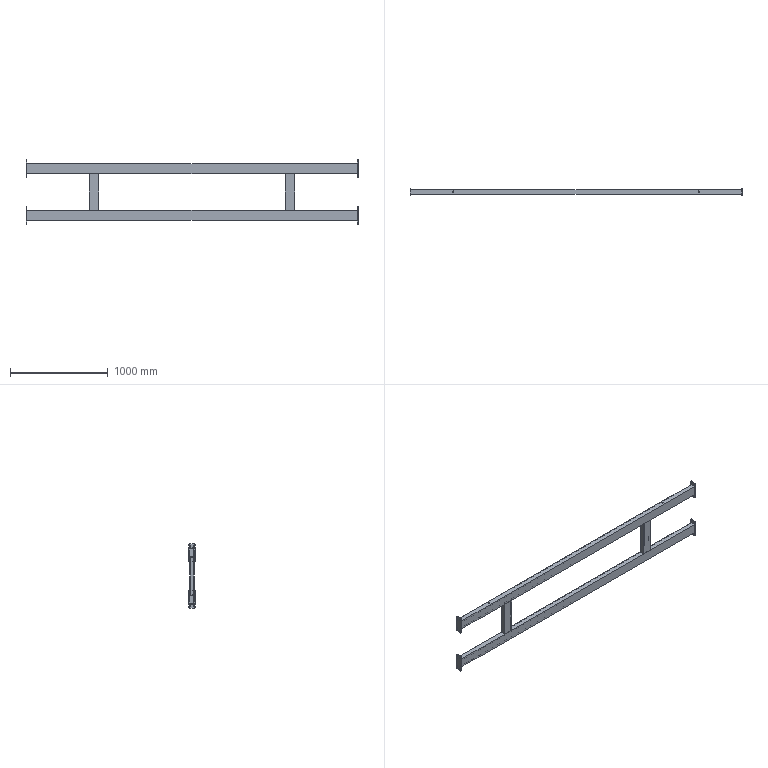Part | SolidWorks | features ICE 2, WeldMemberFeat 2, DelFace 1, MirrorSolid 1, MoveCopyBody 1, PLine 1, WeldCornerFeat 1, WeldmentFeature 1 | 8 solids | 136 faces | box 3391 x 70 x 655 mm | volume 10020196 mm3 | cylinder 68 | plane 68 | commonest cylinder face diameters 14 x32 20 x16 8.4 x8 17 x8 12 x4